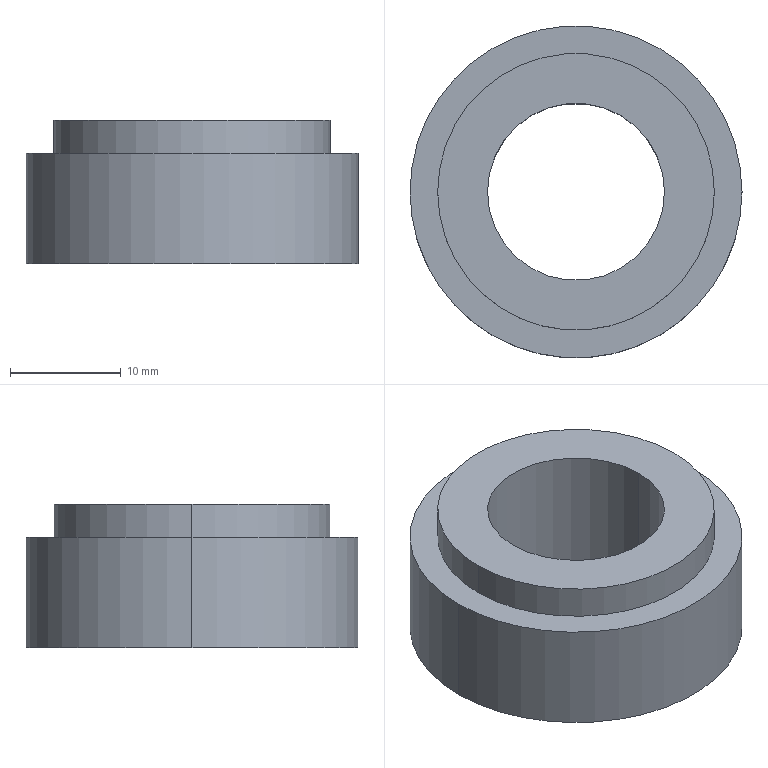Part | SolidWorks | features ICE 2, Extrusion 1 | 1 solid | 9 faces | box 30 x 30 x 13 mm | volume 5927 mm3 | cylinder 6 | plane 3 | commonest cylinder face diameters 16 x2 25 x2 30 x2
STEP:
#1=CARTESIAN_POINT('',(-8.,0.,0.));
#2=VERTEX_POINT('',#1);
#3=CARTESIAN_POINT('',(8.,0.,0.));
#4=VERTEX_POINT('',#3);
#5=CARTESIAN_POINT('',(0.,0.,0.));
#6=DIRECTION('',(0.,0.,1.));
#7=DIRECTION('',(1.,0.,0.));
#8=AXIS2_PLACEMENT_3D('',#5,#6,#7);
#9=CIRCLE('',#8,8.);
#10=EDGE_CURVE('',#2,#4,#9,.T.);
#11=ORIENTED_EDGE('',*,*,#10,.F.);
#12=CARTESIAN_POINT('',(-8.,0.,13.));
#13=VERTEX_POINT('',#12);
#14=CARTESIAN_POINT('',(-8.,0.,0.));
#15=DIRECTION('',(0.,0.,1.));
#16=VECTOR('',#15,1000.);
#17=LINE('',#14,#16);
#18=EDGE_CURVE('',#2,#13,#17,.T.);
#19=ORIENTED_EDGE('',*,*,#18,.T.);
#20=CARTESIAN_POINT('',(8.,0.,13.));
#21=VERTEX_POINT('',#20);
#22=CARTESIAN_POINT('',(0.,0.,13.));
#23=DIRECTION('',(0.,0.,1.));
#24=DIRECTION('',(1.,0.,0.));
#25=AXIS2_PLACEMENT_3D('',#22,#23,#24);
#26=CIRCLE('',#25,8.);
#27=EDGE_CURVE('',#13,#21,#26,.T.);
#28=ORIENTED_EDGE('',*,*,#27,.T.);
#29=CARTESIAN_POINT('',(8.,0.,0.));
#30=DIRECTION('',(0.,0.,1.));
#31=VECTOR('',#30,1000.);
#32=LINE('',#29,#31);
#33=EDGE_CURVE('',#4,#21,#32,.T.);
#34=ORIENTED_EDGE('',*,*,#33,.F.);
#35=EDGE_LOOP('',(#11,#19,#28,#34));
#36=FACE_OUTER_BOUND('',#35,.T.);
#37=CARTESIAN_POINT('',(0.,0.,0.));
#38=DIRECTION('',(0.,0.,1.));
#39=DIRECTION('',(1.,0.,0.));
#40=AXIS2_PLACEMENT_3D('',#37,#38,#39);
#41=CYLINDRICAL_SURFACE('',#40,8.);
#42=ADVANCED_FACE('',(#36),#41,.F.);
#43=CARTESIAN_POINT('',(12.5,0.,13.));
#44=VERTEX_POINT('',#43);
#45=CARTESIAN_POINT('',(-12.5,0.,13.));
#46=VERTEX_POINT('',#45);
#47=CARTESIAN_POINT('',(0.,0.,13.));
#48=DIRECTION('',(0.,0.,1.));
#49=DIRECTION('',(1.,0.,0.));
#50=AXIS2_PLACEMENT_3D('',#47,#48,#49);
#51=CIRCLE('',#50,12.5);
#52=EDGE_CURVE('',#44,#46,#51,.T.);
#53=ORIENTED_EDGE('',*,*,#52,.F.);
#54=CARTESIAN_POINT('',(12.5,0.,10.));
#55=VERTEX_POINT('',#54);
#56=CARTESIAN_POINT('',(12.5,0.,13.));
#57=DIRECTION('',(0.,0.,-1.));
#58=VECTOR('',#57,1000.);
#59=LINE('',#56,#58);
#60=EDGE_CURVE('',#44,#55,#59,.T.);
#61=ORIENTED_EDGE('',*,*,#60,.T.);
#62=CARTESIAN_POINT('',(-12.5,0.,10.));
#63=VERTEX_POINT('',#62);
#64=CARTESIAN_POINT('',(0.,0.,10.));
#65=DIRECTION('',(0.,0.,1.));
#66=DIRECTION('',(1.,0.,0.));
#67=AXIS2_PLACEMENT_3D('',#64,#65,#66);
#68=CIRCLE('',#67,12.5);
#69=EDGE_CURVE('',#55,#63,#68,.T.);
#70=ORIENTED_EDGE('',*,*,#69,.T.);
#71=CARTESIAN_POINT('',(-12.5,0.,13.));
#72=DIRECTION('',(0.,0.,-1.));
#73=VECTOR('',#72,1000.);
#74=LINE('',#71,#73);
#75=EDGE_CURVE('',#46,#63,#74,.T.);
#76=ORIENTED_EDGE('',*,*,#75,.F.);
#77=EDGE_LOOP('',(#53,#61,#70,#76));
#78=FACE_OUTER_BOUND('',#77,.T.);
#79=CARTESIAN_POINT('',(0.,0.,13.));
#80=DIRECTION('',(0.,0.,-1.));
#81=DIRECTION('',(-1.,0.,0.));
#82=AXIS2_PLACEMENT_3D('',#79,#80,#81);
#83=CYLINDRICAL_SURFACE('',#82,12.5);
#84=ADVANCED_FACE('',(#78),#83,.T.);
#85=CARTESIAN_POINT('',(15.,0.,10.));
#86=VERTEX_POINT('',#85);
#87=CARTESIAN_POINT('',(-15.,0.,10.));
#88=VERTEX_POINT('',#87);
#89=CARTESIAN_POINT('',(0.,0.,10.));
#90=DIRECTION('',(0.,0.,1.));
#91=DIRECTION('',(1.,0.,0.));
#92=AXIS2_PLACEMENT_3D('',#89,#90,#91);
#93=CIRCLE('',#92,15.);
#94=EDGE_CURVE('',#86,#88,#93,.T.);
#95=ORIENTED_EDGE('',*,*,#94,.F.);
#96=CARTESIAN_POINT('',(15.,0.,0.));
#97=VERTEX_POINT('',#96);
#98=CARTESIAN_POINT('',(15.,0.,10.));
#99=DIRECTION('',(0.,0.,-1.));
#100=VECTOR('',#99,1000.);
#101=LINE('',#98,#100);
#102=EDGE_CURVE('',#86,#97,#101,.T.);
#103=ORIENTED_EDGE('',*,*,#102,.T.);
#104=CARTESIAN_POINT('',(-15.,0.,0.));
#105=VERTEX_POINT('',#104);
#106=CARTESIAN_POINT('',(0.,0.,0.));
#107=DIRECTION('',(0.,0.,1.));
#108=DIRECTION('',(1.,0.,0.));
#109=AXIS2_PLACEMENT_3D('',#106,#107,#108);
#110=CIRCLE('',#109,15.);
#111=EDGE_CURVE('',#97,#105,#110,.T.);
#112=ORIENTED_EDGE('',*,*,#111,.T.);
#113=CARTESIAN_POINT('',(-15.,0.,10.));
#114=DIRECTION('',(0.,0.,-1.));
#115=VECTOR('',#114,1000.);
#116=LINE('',#113,#115);
#117=EDGE_CURVE('',#88,#105,#116,.T.);
#118=ORIENTED_EDGE('',*,*,#117,.F.);
#119=EDGE_LOOP('',(#95,#103,#112,#118));
#120=FACE_OUTER_BOUND('',#119,.T.);
#121=CARTESIAN_POINT('',(0.,0.,10.));
#122=DIRECTION('',(0.,0.,-1.));
#123=DIRECTION('',(-1.,0.,0.));
#124=AXIS2_PLACEMENT_3D('',#121,#122,#123);
#125=CYLINDRICAL_SURFACE('',#124,15.);
#126=ADVANCED_FACE('',(#120),#125,.T.);
#127=ORIENTED_EDGE('',*,*,#102,.F.);
#128=CARTESIAN_POINT('',(0.,0.,10.));
#129=DIRECTION('',(0.,0.,1.));
#130=DIRECTION('',(1.,0.,0.));
#131=AXIS2_PLACEMENT_3D('',#128,#129,#130);
#132=CIRCLE('',#131,15.);
#133=EDGE_CURVE('',#88,#86,#132,.T.);
#134=ORIENTED_EDGE('',*,*,#133,.F.);
#135=ORIENTED_EDGE('',*,*,#117,.T.);
#136=CARTESIAN_POINT('',(0.,0.,0.));
#137=DIRECTION('',(0.,0.,1.));
#138=DIRECTION('',(1.,0.,0.));
#139=AXIS2_PLACEMENT_3D('',#136,#137,#138);
#140=CIRCLE('',#139,15.);
#141=EDGE_CURVE('',#105,#97,#140,.T.);
#142=ORIENTED_EDGE('',*,*,#141,.T.);
#143=EDGE_LOOP('',(#127,#134,#135,#142));
#144=FACE_OUTER_BOUND('',#143,.T.);
#145=CARTESIAN_POINT('',(0.,0.,10.));
#146=DIRECTION('',(0.,0.,-1.));
#147=DIRECTION('',(-1.,0.,0.));
#148=AXIS2_PLACEMENT_3D('',#145,#146,#147);
#149=CYLINDRICAL_SURFACE('',#148,15.);
#150=ADVANCED_FACE('',(#144),#149,.T.);
#151=CARTESIAN_POINT('',(0.,0.,10.));
#152=DIRECTION('',(0.,0.,1.));
#153=DIRECTION('',(1.,0.,0.));
#154=AXIS2_PLACEMENT_3D('',#151,#152,#153);
#155=CIRCLE('',#154,12.5);
#156=EDGE_CURVE('',#63,#55,#155,.T.);
#157=ORIENTED_EDGE('',*,*,#156,.F.);
#158=ORIENTED_EDGE('',*,*,#69,.F.);
#159=EDGE_LOOP('',(#157,#158));
#160=FACE_BOUND('',#159,.T.);
#161=ORIENTED_EDGE('',*,*,#133,.T.);
#162=ORIENTED_EDGE('',*,*,#94,.T.);
#163=EDGE_LOOP('',(#161,#162));
#164=FACE_OUTER_BOUND('',#163,.T.);
#165=CARTESIAN_POINT('',(0.,0.,10.));
#166=DIRECTION('',(0.,0.,1.));
#167=DIRECTION('',(1.,0.,0.));
#168=AXIS2_PLACEMENT_3D('',#165,#166,#167);
#169=PLANE('',#168);
#170=ADVANCED_FACE('',(#160,#164),#169,.T.);
#171=CARTESIAN_POINT('',(0.,0.,0.));
#172=DIRECTION('',(0.,0.,1.));
#173=DIRECTION('',(1.,0.,0.));
#174=AXIS2_PLACEMENT_3D('',#171,#172,#173);
#175=CIRCLE('',#174,8.);
#176=EDGE_CURVE('',#4,#2,#175,.T.);
#177=ORIENTED_EDGE('',*,*,#176,.T.);
#178=ORIENTED_EDGE('',*,*,#10,.T.);
#179=EDGE_LOOP('',(#177,#178));
#180=FACE_BOUND('',#179,.T.);
#181=ORIENTED_EDGE('',*,*,#141,.F.);
#182=ORIENTED_EDGE('',*,*,#111,.F.);
#183=EDGE_LOOP('',(#181,#182));
#184=FACE_OUTER_BOUND('',#183,.T.);
#185=CARTESIAN_POINT('',(0.,0.,0.));
#186=DIRECTION('',(0.,0.,1.));
#187=DIRECTION('',(1.,0.,0.));
#188=AXIS2_PLACEMENT_3D('',#185,#186,#187);
#189=PLANE('',#188);
#190=ADVANCED_FACE('',(#180,#184),#189,.F.);
#191=ORIENTED_EDGE('',*,*,#60,.F.);
#192=CARTESIAN_POINT('',(0.,0.,13.));
#193=DIRECTION('',(0.,0.,1.));
#194=DIRECTION('',(1.,0.,0.));
#195=AXIS2_PLACEMENT_3D('',#192,#193,#194);
#196=CIRCLE('',#195,12.5);
#197=EDGE_CURVE('',#46,#44,#196,.T.);
#198=ORIENTED_EDGE('',*,*,#197,.F.);
#199=ORIENTED_EDGE('',*,*,#75,.T.);
#200=ORIENTED_EDGE('',*,*,#156,.T.);
#201=EDGE_LOOP('',(#191,#198,#199,#200));
#202=FACE_OUTER_BOUND('',#201,.T.);
#203=CARTESIAN_POINT('',(0.,0.,13.));
#204=DIRECTION('',(0.,0.,-1.));
#205=DIRECTION('',(-1.,0.,0.));
#206=AXIS2_PLACEMENT_3D('',#203,#204,#205);
#207=CYLINDRICAL_SURFACE('',#206,12.5);
#208=ADVANCED_FACE('',(#202),#207,.T.);
#209=CARTESIAN_POINT('',(0.,0.,13.));
#210=DIRECTION('',(0.,0.,1.));
#211=DIRECTION('',(1.,0.,0.));
#212=AXIS2_PLACEMENT_3D('',#209,#210,#211);
#213=CIRCLE('',#212,8.);
#214=EDGE_CURVE('',#21,#13,#213,.T.);
#215=ORIENTED_EDGE('',*,*,#214,.F.);
#216=ORIENTED_EDGE('',*,*,#27,.F.);
#217=EDGE_LOOP('',(#215,#216));
#218=FACE_BOUND('',#217,.T.);
#219=ORIENTED_EDGE('',*,*,#197,.T.);
#220=ORIENTED_EDGE('',*,*,#52,.T.);
#221=EDGE_LOOP('',(#219,#220));
#222=FACE_OUTER_BOUND('',#221,.T.);
#223=CARTESIAN_POINT('',(0.,0.,13.));
#224=DIRECTION('',(0.,0.,1.));
#225=DIRECTION('',(1.,0.,0.));
#226=AXIS2_PLACEMENT_3D('',#223,#224,#225);
#227=PLANE('',#226);
#228=ADVANCED_FACE('',(#218,#222),#227,.T.);
#229=ORIENTED_EDGE('',*,*,#18,.F.);
#230=ORIENTED_EDGE('',*,*,#176,.F.);
#231=ORIENTED_EDGE('',*,*,#33,.T.);
#232=ORIENTED_EDGE('',*,*,#214,.T.);
#233=EDGE_LOOP('',(#229,#230,#231,#232));
#234=FACE_OUTER_BOUND('',#233,.T.);
#235=CARTESIAN_POINT('',(0.,0.,0.));
#236=DIRECTION('',(0.,0.,1.));
#237=DIRECTION('',(1.,0.,0.));
#238=AXIS2_PLACEMENT_3D('',#235,#236,#237);
#239=CYLINDRICAL_SURFACE('',#238,8.);
#240=ADVANCED_FACE('',(#234),#239,.F.);
#241=CLOSED_SHELL('',(#42,#84,#126,#150,#170,#190,#208,#228,#240));
#242=MANIFOLD_SOLID_BREP('',#241);
#243=CARTESIAN_POINT('',(0.,0.,0.));
#244=DIRECTION('',(0.,0.,1.));
#245=DIRECTION('',(1.,0.,0.));
#246=AXIS2_PLACEMENT_3D('',#243,#244,#245);
#247=(LENGTH_UNIT()NAMED_UNIT(*)SI_UNIT(.MILLI.,.METRE.));
#248=UNCERTAINTY_MEASURE_WITH_UNIT(LENGTH_MEASURE(0.00001),#247,'','');
#249=(NAMED_UNIT(*)PLANE_ANGLE_UNIT()SI_UNIT($,.RADIAN.));
#250=(NAMED_UNIT(*)SI_UNIT($,.STERADIAN.)SOLID_ANGLE_UNIT());
#251=(GEOMETRIC_REPRESENTATION_CONTEXT(3)GLOBAL_UNCERTAINTY_ASSIGNED_CONTEXT((#248))GLOBAL_UNIT_ASSIGNED_CONTEXT((#247,#249,#250))REPRESENTATION_CONTEXT('',''));
#252=ADVANCED_BREP_SHAPE_REPRESENTATION('',(#242,#246),#251);